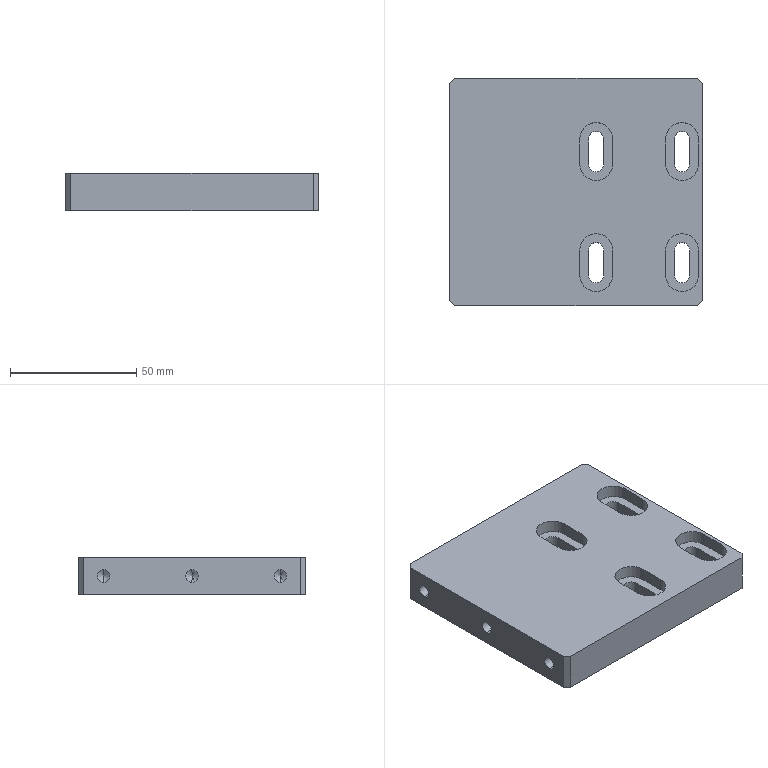Part | SolidWorks | features ICE 2, Chamfer 1, Extrusion 1, HoleWzd 1, LPattern 1 | 1 solid | 58 faces | box 100 x 90 x 15 mm | volume 125181 mm3 | plane 30 | cylinder 22 | cone 6 | commonest cylinder face diameters 6 x8 13 x8 5 x6